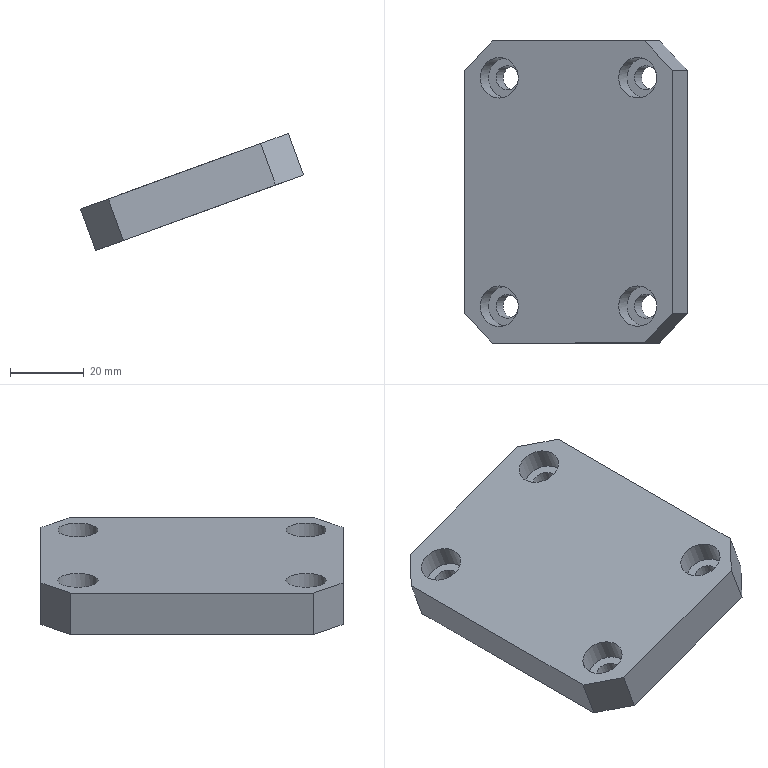Part | STEP file | P011002S003-008 | 1 solid | 22 faces | box 60.486 x 82 x 31.798 mm | volume 54303 mm3 | plane 14 | cylinder 8 | commonest cylinder face diameters 6.5 x4 11 x4